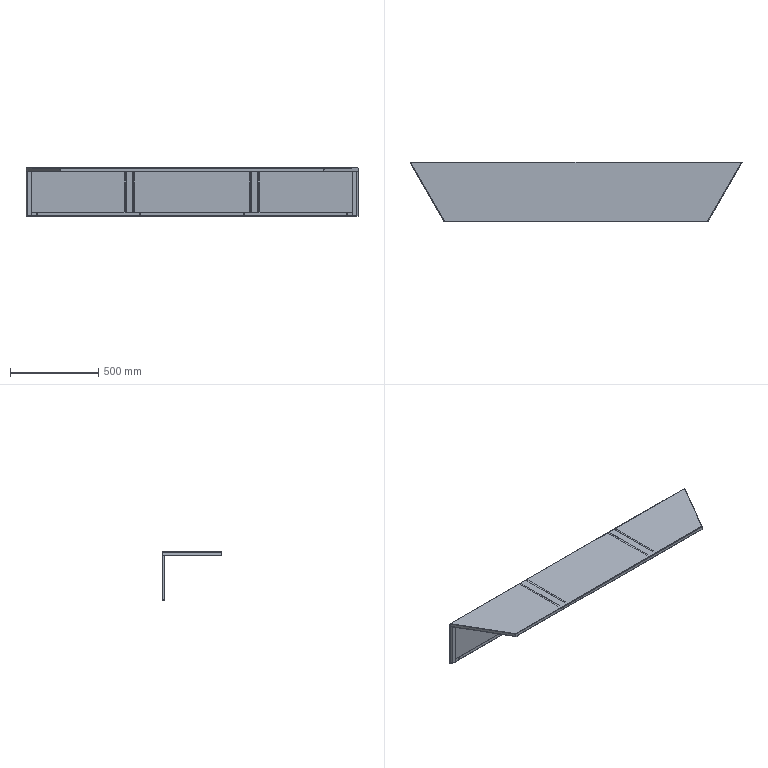Part | SolidWorks | features ReferencePattern 2, LocalLPattern 1 | 7 solids | 347 faces | box 1885 x 336.9 x 273 mm | volume 1993401 mm3 | plane 255 | cylinder 74 | spline 18 | commonest cylinder face diameters 6.4 x20 2 x16 5 x16 1 x11 4 x11